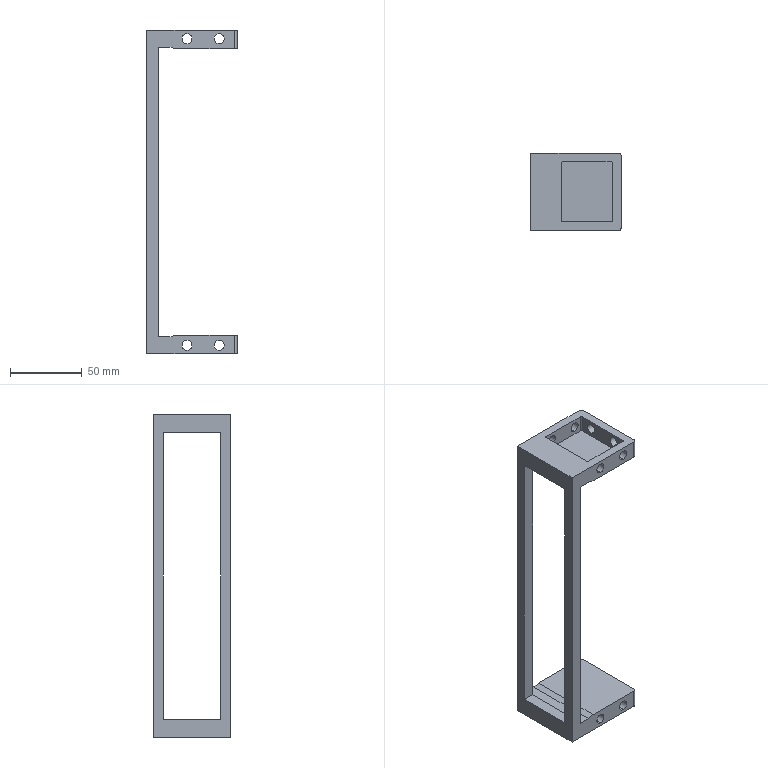Part | STEP file | TKR26H40W200R75+35L-FU-MU-Part-2 | 1 solid | 64 faces | box 63 x 54 x 226 mm | volume 71145 mm3 | cylinder 36 | plane 28 | commonest cylinder face diameters 7 x24 2 x8 4 x4